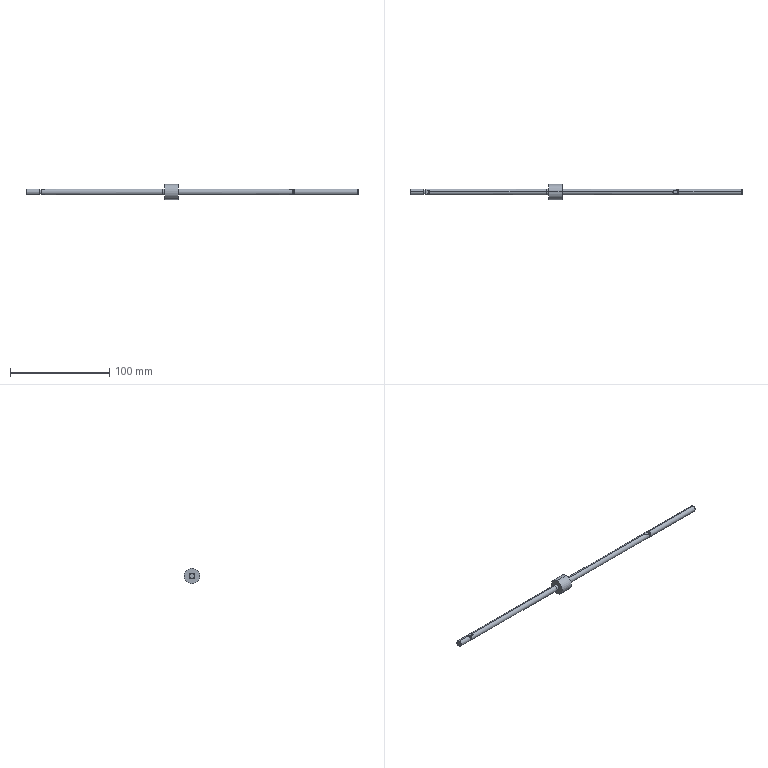Part | SolidWorks | features BaseBody 1 | 1 solid | 41 faces | box 334 x 15.5 x 15.5 mm | volume 11530 mm3 | plane 17 | cylinder 16 | cone 8 | commonest cylinder face diameters 6 x8 4.8 x4 5.8 x2 15.5 x2
STEP:
#1=CARTESIAN_POINT('',(99.1,0.,3.));
#2=VERTEX_POINT('',#1);
#3=CARTESIAN_POINT('',(99.1,0.,-3.));
#4=VERTEX_POINT('',#3);
#5=CARTESIAN_POINT('',(99.1,0.,0.));
#6=DIRECTION('',(-1.,0.,0.));
#7=DIRECTION('',(0.,0.,1.));
#8=AXIS2_PLACEMENT_3D('',#5,#6,#7);
#9=CIRCLE('',#8,3.);
#10=EDGE_CURVE('',#2,#4,#9,.T.);
#11=ORIENTED_EDGE('',*,*,#10,.T.);
#12=CARTESIAN_POINT('',(-18.5,0.,-3.));
#13=VERTEX_POINT('',#12);
#14=CARTESIAN_POINT('',(115.,0.,-3.));
#15=DIRECTION('',(-1.,0.,0.));
#16=VECTOR('',#15,1000.);
#17=LINE('',#14,#16);
#18=EDGE_CURVE('',#4,#13,#17,.T.);
#19=ORIENTED_EDGE('',*,*,#18,.T.);
#20=CARTESIAN_POINT('',(-19.,1.658,-2.5));
#21=VERTEX_POINT('',#20);
#22=CARTESIAN_POINT('',(-18.5,0.,-3.));
#23=CARTESIAN_POINT('',(-18.5,0.5942,-3.));
#24=CARTESIAN_POINT('',(-18.672,1.163,-2.828));
#25=CARTESIAN_POINT('',(-19.,1.658,-2.5));
#26=(BOUNDED_CURVE()B_SPLINE_CURVE(3,(#22,#23,#24,#25),.UNSPECIFIED.,.F.,.F.)B_SPLINE_CURVE_WITH_KNOTS((4,4),(3.142,3.727),.UNSPECIFIED.)CURVE()GEOMETRIC_REPRESENTATION_ITEM()RATIONAL_B_SPLINE_CURVE((1.,0.9716,0.9716,1.))REPRESENTATION_ITEM(''));
#27=EDGE_CURVE('',#13,#21,#26,.T.);
#28=ORIENTED_EDGE('',*,*,#27,.T.);
#29=CARTESIAN_POINT('',(-22.,1.658,-2.5));
#30=VERTEX_POINT('',#29);
#31=CARTESIAN_POINT('',(115.,1.658,-2.5));
#32=DIRECTION('',(-1.,0.,0.));
#33=VECTOR('',#32,1000.);
#34=LINE('',#31,#33);
#35=EDGE_CURVE('',#21,#30,#34,.T.);
#36=ORIENTED_EDGE('',*,*,#35,.T.);
#37=CARTESIAN_POINT('',(-22.,1.658,2.5));
#38=VERTEX_POINT('',#37);
#39=CARTESIAN_POINT('',(-22.,0.,0.));
#40=DIRECTION('',(1.,0.,0.));
#41=DIRECTION('',(0.,0.,1.));
#42=AXIS2_PLACEMENT_3D('',#39,#40,#41);
#43=CIRCLE('',#42,3.);
#44=EDGE_CURVE('',#30,#38,#43,.T.);
#45=ORIENTED_EDGE('',*,*,#44,.T.);
#46=CARTESIAN_POINT('',(-19.,1.658,2.5));
#47=VERTEX_POINT('',#46);
#48=CARTESIAN_POINT('',(115.,1.658,2.5));
#49=DIRECTION('',(1.,0.,0.));
#50=VECTOR('',#49,1000.);
#51=LINE('',#48,#50);
#52=EDGE_CURVE('',#38,#47,#51,.T.);
#53=ORIENTED_EDGE('',*,*,#52,.T.);
#54=CARTESIAN_POINT('',(-18.5,0.,3.));
#55=VERTEX_POINT('',#54);
#56=CARTESIAN_POINT('',(-19.,1.658,2.5));
#57=CARTESIAN_POINT('',(-18.672,1.163,2.828));
#58=CARTESIAN_POINT('',(-18.5,0.5942,3.));
#59=CARTESIAN_POINT('',(-18.5,0.,3.));
#60=(BOUNDED_CURVE()B_SPLINE_CURVE(3,(#56,#57,#58,#59),.UNSPECIFIED.,.F.,.T.)B_SPLINE_CURVE_WITH_KNOTS((4,4),(2.556,3.142),.UNSPECIFIED.)CURVE()GEOMETRIC_REPRESENTATION_ITEM()RATIONAL_B_SPLINE_CURVE((1.,0.9716,0.9716,1.))REPRESENTATION_ITEM(''));
#61=EDGE_CURVE('',#47,#55,#60,.T.);
#62=ORIENTED_EDGE('',*,*,#61,.T.);
#63=CARTESIAN_POINT('',(115.,0.,3.));
#64=DIRECTION('',(-1.,0.,0.));
#65=VECTOR('',#64,1000.);
#66=LINE('',#63,#65);
#67=EDGE_CURVE('',#2,#55,#66,.T.);
#68=ORIENTED_EDGE('',*,*,#67,.F.);
#69=EDGE_LOOP('',(#11,#19,#28,#36,#45,#53,#62,#68));
#70=FACE_OUTER_BOUND('',#69,.T.);
#71=CARTESIAN_POINT('',(115.,0.,0.));
#72=DIRECTION('',(-1.,0.,0.));
#73=DIRECTION('',(0.,0.,1.));
#74=AXIS2_PLACEMENT_3D('',#71,#72,#73);
#75=CYLINDRICAL_SURFACE('',#74,3.);
#76=ADVANCED_FACE('',(#70),#75,.T.);
#77=CARTESIAN_POINT('',(-22.6,0.,-2.4));
#78=VERTEX_POINT('',#77);
#79=CARTESIAN_POINT('',(-22.6,0.,2.4));
#80=VERTEX_POINT('',#79);
#81=CARTESIAN_POINT('',(-22.6,0.,0.));
#82=DIRECTION('',(1.,0.,0.));
#83=DIRECTION('',(0.,0.,-1.));
#84=AXIS2_PLACEMENT_3D('',#81,#82,#83);
#85=CIRCLE('',#84,2.4);
#86=EDGE_CURVE('',#78,#80,#85,.T.);
#87=ORIENTED_EDGE('',*,*,#86,.T.);
#88=CARTESIAN_POINT('',(-22.46,0.,2.54));
#89=VERTEX_POINT('',#88);
#90=CARTESIAN_POINT('',(-22.,0.,3.));
#91=DIRECTION('',(0.7071,0.,0.7071));
#92=VECTOR('',#91,1000.);
#93=LINE('',#90,#92);
#94=EDGE_CURVE('',#80,#89,#93,.T.);
#95=ORIENTED_EDGE('',*,*,#94,.T.);
#96=CARTESIAN_POINT('',(-22.46,0.449,2.5));
#97=VERTEX_POINT('',#96);
#98=CARTESIAN_POINT('',(-22.46,0.,0.));
#99=DIRECTION('',(-1.,0.,0.));
#100=DIRECTION('',(0.,0.,-1.));
#101=AXIS2_PLACEMENT_3D('',#98,#99,#100);
#102=CIRCLE('',#101,2.54);
#103=EDGE_CURVE('',#89,#97,#102,.T.);
#104=ORIENTED_EDGE('',*,*,#103,.T.);
#105=CARTESIAN_POINT('',(-22.,1.658,2.5));
#106=CARTESIAN_POINT('',(-22.211,1.277,2.5));
#107=CARTESIAN_POINT('',(-22.384,0.8814,2.5));
#108=CARTESIAN_POINT('',(-22.46,0.449,2.5));
#109=B_SPLINE_CURVE_WITH_KNOTS('',3,(#105,#106,#107,#108),.UNSPECIFIED.,.F.,.F.,(4,4),(0.,0.001294),.UNSPECIFIED.);
#110=EDGE_CURVE('',#38,#97,#109,.T.);
#111=ORIENTED_EDGE('',*,*,#110,.F.);
#112=ORIENTED_EDGE('',*,*,#44,.F.);
#113=CARTESIAN_POINT('',(-22.46,0.449,-2.5));
#114=VERTEX_POINT('',#113);
#115=CARTESIAN_POINT('',(-22.,1.658,-2.5));
#116=CARTESIAN_POINT('',(-22.211,1.277,-2.5));
#117=CARTESIAN_POINT('',(-22.384,0.8814,-2.5));
#118=CARTESIAN_POINT('',(-22.46,0.449,-2.5));
#119=B_SPLINE_CURVE_WITH_KNOTS('',3,(#115,#116,#117,#118),.UNSPECIFIED.,.F.,.F.,(4,4),(0.,0.001294),.UNSPECIFIED.);
#120=EDGE_CURVE('',#30,#114,#119,.T.);
#121=ORIENTED_EDGE('',*,*,#120,.T.);
#122=CARTESIAN_POINT('',(-22.46,0.,-2.54));
#123=VERTEX_POINT('',#122);
#124=CARTESIAN_POINT('',(-22.46,0.,0.));
#125=DIRECTION('',(-1.,0.,0.));
#126=DIRECTION('',(0.,0.,-1.));
#127=AXIS2_PLACEMENT_3D('',#124,#125,#126);
#128=CIRCLE('',#127,2.54);
#129=EDGE_CURVE('',#114,#123,#128,.T.);
#130=ORIENTED_EDGE('',*,*,#129,.T.);
#131=CARTESIAN_POINT('',(-22.,0.,-3.));
#132=DIRECTION('',(0.7071,0.,-0.7071));
#133=VECTOR('',#132,1000.);
#134=LINE('',#131,#133);
#135=EDGE_CURVE('',#78,#123,#134,.T.);
#136=ORIENTED_EDGE('',*,*,#135,.F.);
#137=EDGE_LOOP('',(#87,#95,#104,#111,#112,#121,#130,#136));
#138=FACE_OUTER_BOUND('',#137,.T.);
#139=CARTESIAN_POINT('',(-22.,0.,0.));
#140=DIRECTION('',(1.,0.,0.));
#141=DIRECTION('',(0.,0.,-1.));
#142=AXIS2_PLACEMENT_3D('',#139,#140,#141);
#143=CONICAL_SURFACE('',#142,3.,0.7854);
#144=ADVANCED_FACE('',(#138),#143,.T.);
#145=ORIENTED_EDGE('',*,*,#86,.F.);
#146=CARTESIAN_POINT('',(-24.,0.,-2.4));
#147=VERTEX_POINT('',#146);
#148=CARTESIAN_POINT('',(115.,0.,-2.4));
#149=DIRECTION('',(-1.,0.,0.));
#150=VECTOR('',#149,1000.);
#151=LINE('',#148,#150);
#152=EDGE_CURVE('',#78,#147,#151,.T.);
#153=ORIENTED_EDGE('',*,*,#152,.T.);
#154=CARTESIAN_POINT('',(-24.,0.,2.4));
#155=VERTEX_POINT('',#154);
#156=CARTESIAN_POINT('',(-24.,0.,0.));
#157=DIRECTION('',(1.,0.,0.));
#158=DIRECTION('',(0.,0.,1.));
#159=AXIS2_PLACEMENT_3D('',#156,#157,#158);
#160=CIRCLE('',#159,2.4);
#161=EDGE_CURVE('',#147,#155,#160,.T.);
#162=ORIENTED_EDGE('',*,*,#161,.T.);
#163=CARTESIAN_POINT('',(115.,0.,2.4));
#164=DIRECTION('',(-1.,0.,0.));
#165=VECTOR('',#164,1000.);
#166=LINE('',#163,#165);
#167=EDGE_CURVE('',#80,#155,#166,.T.);
#168=ORIENTED_EDGE('',*,*,#167,.F.);
#169=EDGE_LOOP('',(#145,#153,#162,#168));
#170=FACE_OUTER_BOUND('',#169,.T.);
#171=CARTESIAN_POINT('',(115.,0.,0.));
#172=DIRECTION('',(-1.,0.,0.));
#173=DIRECTION('',(0.,0.,1.));
#174=AXIS2_PLACEMENT_3D('',#171,#172,#173);
#175=CYLINDRICAL_SURFACE('',#174,2.4);
#176=ADVANCED_FACE('',(#170),#175,.T.);
#177=CARTESIAN_POINT('',(101.6,0.,2.9));
#178=VERTEX_POINT('',#177);
#179=CARTESIAN_POINT('',(101.6,0.,-2.9));
#180=VERTEX_POINT('',#179);
#181=CARTESIAN_POINT('',(101.6,0.,0.));
#182=DIRECTION('',(-1.,0.,0.));
#183=DIRECTION('',(0.,0.,1.));
#184=AXIS2_PLACEMENT_3D('',#181,#182,#183);
#185=CIRCLE('',#184,2.9);
#186=EDGE_CURVE('',#178,#180,#185,.T.);
#187=ORIENTED_EDGE('',*,*,#186,.T.);
#188=CARTESIAN_POINT('',(99.1,0.,-2.9));
#189=VERTEX_POINT('',#188);
#190=CARTESIAN_POINT('',(115.,0.,-2.9));
#191=DIRECTION('',(-1.,0.,0.));
#192=VECTOR('',#191,1000.);
#193=LINE('',#190,#192);
#194=EDGE_CURVE('',#180,#189,#193,.T.);
#195=ORIENTED_EDGE('',*,*,#194,.T.);
#196=CARTESIAN_POINT('',(99.1,0.,2.9));
#197=VERTEX_POINT('',#196);
#198=CARTESIAN_POINT('',(99.1,0.,0.));
#199=DIRECTION('',(1.,0.,0.));
#200=DIRECTION('',(0.,0.,1.));
#201=AXIS2_PLACEMENT_3D('',#198,#199,#200);
#202=CIRCLE('',#201,2.9);
#203=EDGE_CURVE('',#189,#197,#202,.T.);
#204=ORIENTED_EDGE('',*,*,#203,.T.);
#205=CARTESIAN_POINT('',(115.,0.,2.9));
#206=DIRECTION('',(-1.,0.,0.));
#207=VECTOR('',#206,1000.);
#208=LINE('',#205,#207);
#209=EDGE_CURVE('',#178,#197,#208,.T.);
#210=ORIENTED_EDGE('',*,*,#209,.F.);
#211=EDGE_LOOP('',(#187,#195,#204,#210));
#212=FACE_OUTER_BOUND('',#211,.T.);
#213=CARTESIAN_POINT('',(115.,0.,0.));
#214=DIRECTION('',(-1.,0.,0.));
#215=DIRECTION('',(0.,0.,1.));
#216=AXIS2_PLACEMENT_3D('',#213,#214,#215);
#217=CYLINDRICAL_SURFACE('',#216,2.9);
#218=ADVANCED_FACE('',(#212),#217,.T.);
#219=CARTESIAN_POINT('',(-24.,0.,3.));
#220=VERTEX_POINT('',#219);
#221=CARTESIAN_POINT('',(-24.,0.,-3.));
#222=VERTEX_POINT('',#221);
#223=CARTESIAN_POINT('',(-24.,0.,0.));
#224=DIRECTION('',(-1.,0.,0.));
#225=DIRECTION('',(0.,0.,1.));
#226=AXIS2_PLACEMENT_3D('',#223,#224,#225);
#227=CIRCLE('',#226,3.);
#228=EDGE_CURVE('',#220,#222,#227,.T.);
#229=ORIENTED_EDGE('',*,*,#228,.T.);
#230=CARTESIAN_POINT('',(-37.387,0.,-3.));
#231=VERTEX_POINT('',#230);
#232=CARTESIAN_POINT('',(115.,0.,-3.));
#233=DIRECTION('',(-1.,0.,0.));
#234=VECTOR('',#233,1000.);
#235=LINE('',#232,#234);
#236=EDGE_CURVE('',#222,#231,#235,.T.);
#237=ORIENTED_EDGE('',*,*,#236,.T.);
#238=CARTESIAN_POINT('',(-37.387,0.,3.));
#239=VERTEX_POINT('',#238);
#240=CARTESIAN_POINT('',(-37.387,0.,0.));
#241=DIRECTION('',(1.,0.,0.));
#242=DIRECTION('',(0.,0.,1.));
#243=AXIS2_PLACEMENT_3D('',#240,#241,#242);
#244=CIRCLE('',#243,3.);
#245=EDGE_CURVE('',#231,#239,#244,.T.);
#246=ORIENTED_EDGE('',*,*,#245,.T.);
#247=CARTESIAN_POINT('',(115.,0.,3.));
#248=DIRECTION('',(-1.,0.,0.));
#249=VECTOR('',#248,1000.);
#250=LINE('',#247,#249);
#251=EDGE_CURVE('',#220,#239,#250,.T.);
#252=ORIENTED_EDGE('',*,*,#251,.F.);
#253=EDGE_LOOP('',(#229,#237,#246,#252));
#254=FACE_OUTER_BOUND('',#253,.T.);
#255=CARTESIAN_POINT('',(115.,0.,0.));
#256=DIRECTION('',(-1.,0.,0.));
#257=DIRECTION('',(0.,0.,1.));
#258=AXIS2_PLACEMENT_3D('',#255,#256,#257);
#259=CYLINDRICAL_SURFACE('',#258,3.);
#260=ADVANCED_FACE('',(#254),#259,.T.);
#261=CARTESIAN_POINT('',(115.,0.,7.75));
#262=VERTEX_POINT('',#261);
#263=CARTESIAN_POINT('',(115.,0.,-7.75));
#264=VERTEX_POINT('',#263);
#265=CARTESIAN_POINT('',(115.,0.,0.));
#266=DIRECTION('',(-1.,0.,0.));
#267=DIRECTION('',(0.,0.,1.));
#268=AXIS2_PLACEMENT_3D('',#265,#266,#267);
#269=CIRCLE('',#268,7.75);
#270=EDGE_CURVE('',#262,#264,#269,.T.);
#271=ORIENTED_EDGE('',*,*,#270,.T.);
#272=CARTESIAN_POINT('',(101.6,0.,-7.75));
#273=VERTEX_POINT('',#272);
#274=CARTESIAN_POINT('',(115.,0.,-7.75));
#275=DIRECTION('',(-1.,0.,0.));
#276=VECTOR('',#275,1000.);
#277=LINE('',#274,#276);
#278=EDGE_CURVE('',#264,#273,#277,.T.);
#279=ORIENTED_EDGE('',*,*,#278,.T.);
#280=CARTESIAN_POINT('',(101.6,0.,7.75));
#281=VERTEX_POINT('',#280);
#282=CARTESIAN_POINT('',(101.6,0.,0.));
#283=DIRECTION('',(1.,0.,0.));
#284=DIRECTION('',(0.,0.,1.));
#285=AXIS2_PLACEMENT_3D('',#282,#283,#284);
#286=CIRCLE('',#285,7.75);
#287=EDGE_CURVE('',#273,#281,#286,.T.);
#288=ORIENTED_EDGE('',*,*,#287,.T.);
#289=CARTESIAN_POINT('',(115.,0.,7.75));
#290=DIRECTION('',(-1.,0.,0.));
#291=VECTOR('',#290,1000.);
#292=LINE('',#289,#291);
#293=EDGE_CURVE('',#262,#281,#292,.T.);
#294=ORIENTED_EDGE('',*,*,#293,.F.);
#295=EDGE_LOOP('',(#271,#279,#288,#294));
#296=FACE_OUTER_BOUND('',#295,.T.);
#297=CARTESIAN_POINT('',(115.,0.,0.));
#298=DIRECTION('',(-1.,0.,0.));
#299=DIRECTION('',(0.,0.,1.));
#300=AXIS2_PLACEMENT_3D('',#297,#298,#299);
#301=CYLINDRICAL_SURFACE('',#300,7.75);
#302=ADVANCED_FACE('',(#296),#301,.T.);
#303=CARTESIAN_POINT('',(-38.,0.,-2.387));
#304=VERTEX_POINT('',#303);
#305=CARTESIAN_POINT('',(-38.,0.,2.387));
#306=VERTEX_POINT('',#305);
#307=CARTESIAN_POINT('',(-38.,0.,0.));
#308=DIRECTION('',(1.,0.,0.));
#309=DIRECTION('',(0.,0.,-1.));
#310=AXIS2_PLACEMENT_3D('',#307,#308,#309);
#311=CIRCLE('',#310,2.387);
#312=EDGE_CURVE('',#304,#306,#311,.T.);
#313=ORIENTED_EDGE('',*,*,#312,.T.);
#314=CARTESIAN_POINT('',(-37.387,0.,3.));
#315=DIRECTION('',(0.7071,0.,0.7071));
#316=VECTOR('',#315,1000.);
#317=LINE('',#314,#316);
#318=EDGE_CURVE('',#306,#239,#317,.T.);
#319=ORIENTED_EDGE('',*,*,#318,.T.);
#320=ORIENTED_EDGE('',*,*,#245,.F.);
#321=CARTESIAN_POINT('',(-37.387,0.,-3.));
#322=DIRECTION('',(0.7071,0.,-0.7071));
#323=VECTOR('',#322,1000.);
#324=LINE('',#321,#323);
#325=EDGE_CURVE('',#304,#231,#324,.T.);
#326=ORIENTED_EDGE('',*,*,#325,.F.);
#327=EDGE_LOOP('',(#313,#319,#320,#326));
#328=FACE_OUTER_BOUND('',#327,.T.);
#329=CARTESIAN_POINT('',(-37.387,0.,0.));
#330=DIRECTION('',(1.,0.,0.));
#331=DIRECTION('',(0.,0.,-1.));
#332=AXIS2_PLACEMENT_3D('',#329,#330,#331);
#333=CONICAL_SURFACE('',#332,3.,0.7854);
#334=ADVANCED_FACE('',(#328),#333,.T.);
#335=CARTESIAN_POINT('',(227.,1.658,-2.5));
#336=VERTEX_POINT('',#335);
#337=CARTESIAN_POINT('',(226.5,0.,-3.));
#338=VERTEX_POINT('',#337);
#339=CARTESIAN_POINT('',(227.,1.658,-2.5));
#340=CARTESIAN_POINT('',(226.672,1.163,-2.828));
#341=CARTESIAN_POINT('',(226.5,0.5942,-3.));
#342=CARTESIAN_POINT('',(226.5,0.,-3.));
#343=(BOUNDED_CURVE()B_SPLINE_CURVE(3,(#339,#340,#341,#342),.UNSPECIFIED.,.F.,.F.)B_SPLINE_CURVE_WITH_KNOTS((4,4),(5.697,6.283),.UNSPECIFIED.)CURVE()GEOMETRIC_REPRESENTATION_ITEM()RATIONAL_B_SPLINE_CURVE((1.,0.9716,0.9716,1.))REPRESENTATION_ITEM(''));
#344=EDGE_CURVE('',#336,#338,#343,.T.);
#345=ORIENTED_EDGE('',*,*,#344,.T.);
#346=CARTESIAN_POINT('',(115.,0.,-3.));
#347=VERTEX_POINT('',#346);
#348=CARTESIAN_POINT('',(296.,0.,-3.));
#349=DIRECTION('',(-1.,0.,0.));
#350=VECTOR('',#349,1000.);
#351=LINE('',#348,#350);
#352=EDGE_CURVE('',#338,#347,#351,.T.);
#353=ORIENTED_EDGE('',*,*,#352,.T.);
#354=CARTESIAN_POINT('',(115.,0.,3.));
#355=VERTEX_POINT('',#354);
#356=CARTESIAN_POINT('',(115.,0.,0.));
#357=DIRECTION('',(1.,0.,0.));
#358=DIRECTION('',(0.,0.,1.));
#359=AXIS2_PLACEMENT_3D('',#356,#357,#358);
#360=CIRCLE('',#359,3.);
#361=EDGE_CURVE('',#347,#355,#360,.T.);
#362=ORIENTED_EDGE('',*,*,#361,.T.);
#363=CARTESIAN_POINT('',(226.5,0.,3.));
#364=VERTEX_POINT('',#363);
#365=CARTESIAN_POINT('',(296.,0.,3.));
#366=DIRECTION('',(-1.,0.,0.));
#367=VECTOR('',#366,1000.);
#368=LINE('',#365,#367);
#369=EDGE_CURVE('',#364,#355,#368,.T.);
#370=ORIENTED_EDGE('',*,*,#369,.F.);
#371=CARTESIAN_POINT('',(227.,1.658,2.5));
#372=VERTEX_POINT('',#371);
#373=CARTESIAN_POINT('',(226.5,0.,3.));
#374=CARTESIAN_POINT('',(226.5,0.5942,3.));
#375=CARTESIAN_POINT('',(226.672,1.163,2.828));
#376=CARTESIAN_POINT('',(227.,1.658,2.5));
#377=(BOUNDED_CURVE()B_SPLINE_CURVE(3,(#373,#374,#375,#376),.UNSPECIFIED.,.F.,.F.)B_SPLINE_CURVE_WITH_KNOTS((4,4),(0.,0.5857),.UNSPECIFIED.)CURVE()GEOMETRIC_REPRESENTATION_ITEM()RATIONAL_B_SPLINE_CURVE((1.,0.9716,0.9716,1.))REPRESENTATION_ITEM(''));
#378=EDGE_CURVE('',#364,#372,#377,.T.);
#379=ORIENTED_EDGE('',*,*,#378,.T.);
#380=CARTESIAN_POINT('',(230.4,1.658,2.5));
#381=VERTEX_POINT('',#380);
#382=CARTESIAN_POINT('',(296.,1.658,2.5));
#383=DIRECTION('',(1.,0.,0.));
#384=VECTOR('',#383,1000.);
#385=LINE('',#382,#384);
#386=EDGE_CURVE('',#372,#381,#385,.T.);
#387=ORIENTED_EDGE('',*,*,#386,.T.);
#388=CARTESIAN_POINT('',(230.4,1.658,-2.5));
#389=VERTEX_POINT('',#388);
#390=CARTESIAN_POINT('',(230.4,0.,0.));
#391=DIRECTION('',(-1.,0.,0.));
#392=DIRECTION('',(0.,0.,1.));
#393=AXIS2_PLACEMENT_3D('',#390,#391,#392);
#394=CIRCLE('',#393,3.);
#395=EDGE_CURVE('',#381,#389,#394,.T.);
#396=ORIENTED_EDGE('',*,*,#395,.T.);
#397=CARTESIAN_POINT('',(296.,1.658,-2.5));
#398=DIRECTION('',(-1.,0.,0.));
#399=VECTOR('',#398,1000.);
#400=LINE('',#397,#399);
#401=EDGE_CURVE('',#389,#336,#400,.T.);
#402=ORIENTED_EDGE('',*,*,#401,.T.);
#403=EDGE_LOOP('',(#345,#353,#362,#370,#379,#387,#396,#402));
#404=FACE_OUTER_BOUND('',#403,.T.);
#405=CARTESIAN_POINT('',(296.,0.,0.));
#406=DIRECTION('',(-1.,0.,0.));
#407=DIRECTION('',(0.,0.,1.));
#408=AXIS2_PLACEMENT_3D('',#405,#406,#407);
#409=CYLINDRICAL_SURFACE('',#408,3.);
#410=ADVANCED_FACE('',(#404),#409,.T.);
#411=CARTESIAN_POINT('',(231.,0.,2.4));
#412=VERTEX_POINT('',#411);
#413=CARTESIAN_POINT('',(231.,0.,-2.4));
#414=VERTEX_POINT('',#413);
#415=CARTESIAN_POINT('',(231.,0.,0.));
#416=DIRECTION('',(-1.,0.,0.));
#417=DIRECTION('',(0.,0.,1.));
#418=AXIS2_PLACEMENT_3D('',#415,#416,#417);
#419=CIRCLE('',#418,2.4);
#420=EDGE_CURVE('',#412,#414,#419,.T.);
#421=ORIENTED_EDGE('',*,*,#420,.T.);
#422=CARTESIAN_POINT('',(230.9,0.,-2.5));
#423=VERTEX_POINT('',#422);
#424=CARTESIAN_POINT('',(230.4,0.,-3.));
#425=DIRECTION('',(-0.7071,0.,-0.7071));
#426=VECTOR('',#425,1000.);
#427=LINE('',#424,#426);
#428=EDGE_CURVE('',#414,#423,#427,.T.);
#429=ORIENTED_EDGE('',*,*,#428,.T.);
#430=CARTESIAN_POINT('',(230.9,0.,-2.5));
#431=CARTESIAN_POINT('',(230.9,0.1452,-2.5));
#432=CARTESIAN_POINT('',(230.887,0.2917,-2.5));
#433=CARTESIAN_POINT('',(230.837,0.5812,-2.5));
#434=CARTESIAN_POINT('',(230.801,0.7221,-2.5));
#435=CARTESIAN_POINT('',(230.666,1.136,-2.5));
#436=CARTESIAN_POINT('',(230.542,1.402,-2.5));
#437=CARTESIAN_POINT('',(230.4,1.658,-2.5));
#438=B_SPLINE_CURVE_WITH_KNOTS('',3,(#430,#431,#432,#433,#434,#435,#436,#437),.UNSPECIFIED.,.F.,.F.,(4,2,2,4),(0.001744,0.002179,0.002615,0.003485),.UNSPECIFIED.);
#439=EDGE_CURVE('',#423,#389,#438,.T.);
#440=ORIENTED_EDGE('',*,*,#439,.T.);
#441=ORIENTED_EDGE('',*,*,#395,.F.);
#442=CARTESIAN_POINT('',(230.9,0.,2.5));
#443=VERTEX_POINT('',#442);
#444=CARTESIAN_POINT('',(230.9,0.,2.5));
#445=CARTESIAN_POINT('',(230.9,0.1452,2.5));
#446=CARTESIAN_POINT('',(230.887,0.2917,2.5));
#447=CARTESIAN_POINT('',(230.837,0.5812,2.5));
#448=CARTESIAN_POINT('',(230.801,0.7221,2.5));
#449=CARTESIAN_POINT('',(230.666,1.136,2.5));
#450=CARTESIAN_POINT('',(230.542,1.402,2.5));
#451=CARTESIAN_POINT('',(230.4,1.658,2.5));
#452=B_SPLINE_CURVE_WITH_KNOTS('',3,(#444,#445,#446,#447,#448,#449,#450,#451),.UNSPECIFIED.,.F.,.F.,(4,2,2,4),(0.001744,0.002179,0.002615,0.003485),.UNSPECIFIED.);
#453=EDGE_CURVE('',#443,#381,#452,.T.);
#454=ORIENTED_EDGE('',*,*,#453,.F.);
#455=CARTESIAN_POINT('',(230.4,0.,3.));
#456=DIRECTION('',(-0.7071,0.,0.7071));
#457=VECTOR('',#456,1000.);
#458=LINE('',#455,#457);
#459=EDGE_CURVE('',#412,#443,#458,.T.);
#460=ORIENTED_EDGE('',*,*,#459,.F.);
#461=EDGE_LOOP('',(#421,#429,#440,#441,#454,#460));
#462=FACE_OUTER_BOUND('',#461,.T.);
#463=CARTESIAN_POINT('',(230.4,0.,0.));
#464=DIRECTION('',(-1.,0.,0.));
#465=DIRECTION('',(0.,0.,1.));
#466=AXIS2_PLACEMENT_3D('',#463,#464,#465);
#467=CONICAL_SURFACE('',#466,3.,0.7854);
#468=ADVANCED_FACE('',(#462),#467,.T.);
#469=CARTESIAN_POINT('',(232.5,0.,2.4));
#470=VERTEX_POINT('',#469);
#471=CARTESIAN_POINT('',(232.5,0.,-2.4));
#472=VERTEX_POINT('',#471);
#473=CARTESIAN_POINT('',(232.5,0.,0.));
#474=DIRECTION('',(-1.,0.,0.));
#475=DIRECTION('',(0.,0.,1.));
#476=AXIS2_PLACEMENT_3D('',#473,#474,#475);
#477=CIRCLE('',#476,2.4);
#478=EDGE_CURVE('',#470,#472,#477,.T.);
#479=ORIENTED_EDGE('',*,*,#478,.T.);
#480=CARTESIAN_POINT('',(296.,0.,-2.4));
#481=DIRECTION('',(-1.,0.,0.));
#482=VECTOR('',#481,1000.);
#483=LINE('',#480,#482);
#484=EDGE_CURVE('',#472,#414,#483,.T.);
#485=ORIENTED_EDGE('',*,*,#484,.T.);
#486=ORIENTED_EDGE('',*,*,#420,.F.);
#487=CARTESIAN_POINT('',(296.,0.,2.4));
#488=DIRECTION('',(-1.,0.,0.));
#489=VECTOR('',#488,1000.);
#490=LINE('',#487,#489);
#491=EDGE_CURVE('',#470,#412,#490,.T.);
#492=ORIENTED_EDGE('',*,*,#491,.F.);
#493=EDGE_LOOP('',(#479,#485,#486,#492));
#494=FACE_OUTER_BOUND('',#493,.T.);
#495=CARTESIAN_POINT('',(296.,0.,0.));
#496=DIRECTION('',(-1.,0.,0.));
#497=DIRECTION('',(0.,0.,1.));
#498=AXIS2_PLACEMENT_3D('',#495,#496,#497);
#499=CYLINDRICAL_SURFACE('',#498,2.4);
#500=ADVANCED_FACE('',(#494),#499,.T.);
#501=CARTESIAN_POINT('',(295.387,0.,3.));
#502=VERTEX_POINT('',#501);
#503=CARTESIAN_POINT('',(295.387,0.,-3.));
#504=VERTEX_POINT('',#503);
#505=CARTESIAN_POINT('',(295.387,0.,0.));
#506=DIRECTION('',(-1.,0.,0.));
#507=DIRECTION('',(0.,0.,1.));
#508=AXIS2_PLACEMENT_3D('',#505,#506,#507);
#509=CIRCLE('',#508,3.);
#510=EDGE_CURVE('',#502,#504,#509,.T.);
#511=ORIENTED_EDGE('',*,*,#510,.T.);
#512=CARTESIAN_POINT('',(232.5,0.,-3.));
#513=VERTEX_POINT('',#512);
#514=CARTESIAN_POINT('',(296.,0.,-3.));
#515=DIRECTION('',(-1.,0.,0.));
#516=VECTOR('',#515,1000.);
#517=LINE('',#514,#516);
#518=EDGE_CURVE('',#504,#513,#517,.T.);
#519=ORIENTED_EDGE('',*,*,#518,.T.);
#520=CARTESIAN_POINT('',(232.5,0.,3.));
#521=VERTEX_POINT('',#520);
#522=CARTESIAN_POINT('',(232.5,0.,0.));
#523=DIRECTION('',(1.,0.,0.));
#524=DIRECTION('',(0.,0.,1.));
#525=AXIS2_PLACEMENT_3D('',#522,#523,#524);
#526=CIRCLE('',#525,3.);
#527=EDGE_CURVE('',#513,#521,#526,.T.);
#528=ORIENTED_EDGE('',*,*,#527,.T.);
#529=CARTESIAN_POINT('',(296.,0.,3.));
#530=DIRECTION('',(-1.,0.,0.));
#531=VECTOR('',#530,1000.);
#532=LINE('',#529,#531);
#533=EDGE_CURVE('',#502,#521,#532,.T.);
#534=ORIENTED_EDGE('',*,*,#533,.F.);
#535=EDGE_LOOP('',(#511,#519,#528,#534));
#536=FACE_OUTER_BOUND('',#535,.T.);
#537=CARTESIAN_POINT('',(296.,0.,0.));
#538=DIRECTION('',(-1.,0.,0.));
#539=DIRECTION('',(0.,0.,1.));
#540=AXIS2_PLACEMENT_3D('',#537,#538,#539);
#541=CYLINDRICAL_SURFACE('',#540,3.);
#542=ADVANCED_FACE('',(#536),#541,.T.);
#543=CARTESIAN_POINT('',(296.,0.,2.386));
#544=VERTEX_POINT('',#543);
#545=CARTESIAN_POINT('',(296.,0.,-2.386));
#546=VERTEX_POINT('',#545);
#547=CARTESIAN_POINT('',(296.,0.,0.));
#548=DIRECTION('',(-1.,0.,0.));
#549=DIRECTION('',(0.,0.,1.));
#550=AXIS2_PLACEMENT_3D('',#547,#548,#549);
#551=CIRCLE('',#550,2.386);
#552=EDGE_CURVE('',#544,#546,#551,.T.);
#553=ORIENTED_EDGE('',*,*,#552,.T.);
#554=CARTESIAN_POINT('',(295.386,0.,-3.));
#555=DIRECTION('',(-0.7071,0.,-0.7071));
#556=VECTOR('',#555,1000.);
#557=LINE('',#554,#556);
#558=EDGE_CURVE('',#546,#504,#557,.T.);
#559=ORIENTED_EDGE('',*,*,#558,.T.);
#560=ORIENTED_EDGE('',*,*,#510,.F.);
#561=CARTESIAN_POINT('',(295.386,0.,3.));
#562=DIRECTION('',(-0.7071,0.,0.7071));
#563=VECTOR('',#562,1000.);
#564=LINE('',#561,#563);
#565=EDGE_CURVE('',#544,#502,#564,.T.);
#566=ORIENTED_EDGE('',*,*,#565,.F.);
#567=EDGE_LOOP('',(#553,#559,#560,#566));
#568=FACE_OUTER_BOUND('',#567,.T.);
#569=CARTESIAN_POINT('',(295.386,0.,0.));
#570=DIRECTION('',(-1.,0.,0.));
#571=DIRECTION('',(0.,0.,1.));
#572=AXIS2_PLACEMENT_3D('',#569,#570,#571);
#573=CONICAL_SURFACE('',#572,3.,0.7854);
#574=ADVANCED_FACE('',(#568),#573,.T.);
#575=ORIENTED_EDGE('',*,*,#18,.F.);
#576=CARTESIAN_POINT('',(99.1,0.,0.));
#577=DIRECTION('',(-1.,0.,0.));
#578=DIRECTION('',(0.,0.,1.));
#579=AXIS2_PLACEMENT_3D('',#576,#577,#578);
#580=CIRCLE('',#579,3.);
#581=EDGE_CURVE('',#4,#2,#580,.T.);
#582=ORIENTED_EDGE('',*,*,#581,.T.);
#583=ORIENTED_EDGE('',*,*,#67,.T.);
#584=CARTESIAN_POINT('',(-19.,-1.658,2.5));
#585=VERTEX_POINT('',#584);
#586=CARTESIAN_POINT('',(-18.5,0.,3.));
#587=CARTESIAN_POINT('',(-18.5,-0.5942,3.));
#588=CARTESIAN_POINT('',(-18.672,-1.163,2.828));
#589=CARTESIAN_POINT('',(-19.,-1.658,2.5));
#590=(BOUNDED_CURVE()B_SPLINE_CURVE(3,(#586,#587,#588,#589),.UNSPECIFIED.,.F.,.F.)B_SPLINE_CURVE_WITH_KNOTS((4,4),(3.142,3.727),.UNSPECIFIED.)CURVE()GEOMETRIC_REPRESENTATION_ITEM()RATIONAL_B_SPLINE_CURVE((1.,0.9716,0.9716,1.))REPRESENTATION_ITEM(''));
#591=EDGE_CURVE('',#55,#585,#590,.T.);
#592=ORIENTED_EDGE('',*,*,#591,.T.);
#593=CARTESIAN_POINT('',(-22.,-1.658,2.5));
#594=VERTEX_POINT('',#593);
#595=CARTESIAN_POINT('',(115.,-1.658,2.5));
#596=DIRECTION('',(-1.,0.,0.));
#597=VECTOR('',#596,1000.);
#598=LINE('',#595,#597);
#599=EDGE_CURVE('',#585,#594,#598,.T.);
#600=ORIENTED_EDGE('',*,*,#599,.T.);
#601=CARTESIAN_POINT('',(-22.,-1.658,-2.5));
#602=VERTEX_POINT('',#601);
#603=CARTESIAN_POINT('',(-22.,0.,0.));
#604=DIRECTION('',(1.,0.,0.));
#605=DIRECTION('',(0.,0.,1.));
#606=AXIS2_PLACEMENT_3D('',#603,#604,#605);
#607=CIRCLE('',#606,3.);
#608=EDGE_CURVE('',#594,#602,#607,.T.);
#609=ORIENTED_EDGE('',*,*,#608,.T.);
#610=CARTESIAN_POINT('',(-19.,-1.658,-2.5));
#611=VERTEX_POINT('',#610);
#612=CARTESIAN_POINT('',(115.,-1.658,-2.5));
#613=DIRECTION('',(1.,0.,0.));
#614=VECTOR('',#613,1000.);
#615=LINE('',#612,#614);
#616=EDGE_CURVE('',#602,#611,#615,.T.);
#617=ORIENTED_EDGE('',*,*,#616,.T.);
#618=CARTESIAN_POINT('',(-19.,-1.658,-2.5));
#619=CARTESIAN_POINT('',(-18.672,-1.163,-2.828));
#620=CARTESIAN_POINT('',(-18.5,-0.5942,-3.));
#621=CARTESIAN_POINT('',(-18.5,0.,-3.));
#622=(BOUNDED_CURVE()B_SPLINE_CURVE(3,(#618,#619,#620,#621),.UNSPECIFIED.,.F.,.F.)B_SPLINE_CURVE_WITH_KNOTS((4,4),(2.556,3.142),.UNSPECIFIED.)CURVE()GEOMETRIC_REPRESENTATION_ITEM()RATIONAL_B_SPLINE_CURVE((1.,0.9716,0.9716,1.))REPRESENTATION_ITEM(''));
#623=EDGE_CURVE('',#611,#13,#622,.T.);
#624=ORIENTED_EDGE('',*,*,#623,.T.);
#625=EDGE_LOOP('',(#575,#582,#583,#592,#600,#609,#617,#624));
#626=FACE_OUTER_BOUND('',#625,.T.);
#627=CARTESIAN_POINT('',(115.,0.,0.));
#628=DIRECTION('',(-1.,0.,0.));
#629=DIRECTION('',(0.,0.,1.));
#630=AXIS2_PLACEMENT_3D('',#627,#628,#629);
#631=CYLINDRICAL_SURFACE('',#630,3.);
#632=ADVANCED_FACE('',(#626),#631,.T.);
#633=ORIENTED_EDGE('',*,*,#61,.F.);
#634=CARTESIAN_POINT('',(-19.,6.,2.5));
#635=DIRECTION('',(0.,-1.,0.));
#636=VECTOR('',#635,1000.);
#637=LINE('',#634,#636);
#638=EDGE_CURVE('',#47,#585,#637,.T.);
#639=ORIENTED_EDGE('',*,*,#638,.T.);
#640=ORIENTED_EDGE('',*,*,#591,.F.);
#641=EDGE_LOOP('',(#633,#639,#640));
#642=FACE_OUTER_BOUND('',#641,.T.);
#643=CARTESIAN_POINT('',(-16.5,6.,5.));
#644=DIRECTION('',(-0.7071,0.,0.7071));
#645=DIRECTION('',(0.7071,0.,0.7071));
#646=AXIS2_PLACEMENT_3D('',#643,#644,#645);
#647=PLANE('',#646);
#648=ADVANCED_FACE('',(#642),#647,.T.);
#649=ORIENTED_EDGE('',*,*,#110,.T.);
#650=CARTESIAN_POINT('',(-22.46,-0.449,2.5));
#651=VERTEX_POINT('',#650);
#652=CARTESIAN_POINT('',(-22.46,6.,2.5));
#653=DIRECTION('',(0.,-1.,0.));
#654=VECTOR('',#653,1000.);
#655=LINE('',#652,#654);
#656=EDGE_CURVE('',#97,#651,#655,.T.);
#657=ORIENTED_EDGE('',*,*,#656,.T.);
#658=CARTESIAN_POINT('',(-22.46,-0.449,2.5));
#659=CARTESIAN_POINT('',(-22.384,-0.8798,2.5));
#660=CARTESIAN_POINT('',(-22.211,-1.277,2.5));
#661=CARTESIAN_POINT('',(-22.,-1.658,2.5));
#662=B_SPLINE_CURVE_WITH_KNOTS('',3,(#658,#659,#660,#661),.UNSPECIFIED.,.F.,.F.,(4,4),(0.,0.001294),.UNSPECIFIED.);
#663=EDGE_CURVE('',#651,#594,#662,.T.);
#664=ORIENTED_EDGE('',*,*,#663,.T.);
#665=ORIENTED_EDGE('',*,*,#599,.F.);
#666=ORIENTED_EDGE('',*,*,#638,.F.);
#667=ORIENTED_EDGE('',*,*,#52,.F.);
#668=EDGE_LOOP('',(#649,#657,#664,#665,#666,#667));
#669=FACE_OUTER_BOUND('',#668,.T.);
#670=CARTESIAN_POINT('',(-19.,6.,2.5));
#671=DIRECTION('',(0.,0.,1.));
#672=DIRECTION('',(1.,0.,0.));
#673=AXIS2_PLACEMENT_3D('',#670,#671,#672);
#674=PLANE('',#673);
#675=ADVANCED_FACE('',(#669),#674,.T.);
#676=ORIENTED_EDGE('',*,*,#94,.F.);
#677=CARTESIAN_POINT('',(-22.6,0.,0.));
#678=DIRECTION('',(1.,0.,0.));
#679=DIRECTION('',(0.,0.,-1.));
#680=AXIS2_PLACEMENT_3D('',#677,#678,#679);
#681=CIRCLE('',#680,2.4);
#682=EDGE_CURVE('',#80,#78,#681,.T.);
#683=ORIENTED_EDGE('',*,*,#682,.T.);
#684=ORIENTED_EDGE('',*,*,#135,.T.);
#685=CARTESIAN_POINT('',(-22.46,-0.449,-2.5));
#686=VERTEX_POINT('',#685);
#687=CARTESIAN_POINT('',(-22.46,0.,0.));
#688=DIRECTION('',(-1.,0.,0.));
#689=DIRECTION('',(0.,0.,-1.));
#690=AXIS2_PLACEMENT_3D('',#687,#688,#689);
#691=CIRCLE('',#690,2.54);
#692=EDGE_CURVE('',#123,#686,#691,.T.);
#693=ORIENTED_EDGE('',*,*,#692,.T.);
#694=CARTESIAN_POINT('',(-22.46,-0.449,-2.5));
#695=CARTESIAN_POINT('',(-22.384,-0.8798,-2.5));
#696=CARTESIAN_POINT('',(-22.211,-1.277,-2.5));
#697=CARTESIAN_POINT('',(-22.,-1.658,-2.5));
#698=B_SPLINE_CURVE_WITH_KNOTS('',3,(#694,#695,#696,#697),.UNSPECIFIED.,.F.,.F.,(4,4),(0.,0.001294),.UNSPECIFIED.);
#699=EDGE_CURVE('',#686,#602,#698,.T.);
#700=ORIENTED_EDGE('',*,*,#699,.T.);
#701=ORIENTED_EDGE('',*,*,#608,.F.);
#702=ORIENTED_EDGE('',*,*,#663,.F.);
#703=CARTESIAN_POINT('',(-22.46,0.,0.));
#704=DIRECTION('',(-1.,0.,0.));
#705=DIRECTION('',(0.,0.,-1.));
#706=AXIS2_PLACEMENT_3D('',#703,#704,#705);
#707=CIRCLE('',#706,2.54);
#708=EDGE_CURVE('',#651,#89,#707,.T.);
#709=ORIENTED_EDGE('',*,*,#708,.T.);
#710=EDGE_LOOP('',(#676,#683,#684,#693,#700,#701,#702,#709));
#711=FACE_OUTER_BOUND('',#710,.T.);
#712=CARTESIAN_POINT('',(-22.,0.,0.));
#713=DIRECTION('',(1.,0.,0.));
#714=DIRECTION('',(0.,0.,-1.));
#715=AXIS2_PLACEMENT_3D('',#712,#713,#714);
#716=CONICAL_SURFACE('',#715,3.,0.7854);
#717=ADVANCED_FACE('',(#711),#716,.T.);
#718=ORIENTED_EDGE('',*,*,#699,.F.);
#719=CARTESIAN_POINT('',(-22.46,6.,-2.5));
#720=DIRECTION('',(0.,1.,0.));
#721=VECTOR('',#720,1000.);
#722=LINE('',#719,#721);
#723=EDGE_CURVE('',#686,#114,#722,.T.);
#724=ORIENTED_EDGE('',*,*,#723,.T.);
#725=ORIENTED_EDGE('',*,*,#120,.F.);
#726=ORIENTED_EDGE('',*,*,#35,.F.);
#727=CARTESIAN_POINT('',(-19.,6.,-2.5));
#728=DIRECTION('',(0.,-1.,0.));
#729=VECTOR('',#728,1000.);
#730=LINE('',#727,#729);
#731=EDGE_CURVE('',#21,#611,#730,.T.);
#732=ORIENTED_EDGE('',*,*,#731,.T.);
#733=ORIENTED_EDGE('',*,*,#616,.F.);
#734=EDGE_LOOP('',(#718,#724,#725,#726,#732,#733));
#735=FACE_OUTER_BOUND('',#734,.T.);
#736=CARTESIAN_POINT('',(-22.46,6.,-2.5));
#737=DIRECTION('',(0.,0.,-1.));
#738=DIRECTION('',(-1.,0.,0.));
#739=AXIS2_PLACEMENT_3D('',#736,#737,#738);
#740=PLANE('',#739);
#741=ADVANCED_FACE('',(#735),#740,.T.);
#742=ORIENTED_EDGE('',*,*,#623,.F.);
#743=ORIENTED_EDGE('',*,*,#731,.F.);
#744=ORIENTED_EDGE('',*,*,#27,.F.);
#745=EDGE_LOOP('',(#742,#743,#744));
#746=FACE_OUTER_BOUND('',#745,.T.);
#747=CARTESIAN_POINT('',(-19.,6.,-2.5));
#748=DIRECTION('',(-0.7071,0.,-0.7071));
#749=DIRECTION('',(-0.7071,0.,0.7071));
#750=AXIS2_PLACEMENT_3D('',#747,#748,#749);
#751=PLANE('',#750);
#752=ADVANCED_FACE('',(#746),#751,.T.);
#753=ORIENTED_EDGE('',*,*,#10,.F.);
#754=ORIENTED_EDGE('',*,*,#581,.F.);
#755=EDGE_LOOP('',(#753,#754));
#756=FACE_OUTER_BOUND('',#755,.T.);
#757=CARTESIAN_POINT('',(99.1,0.,0.));
#758=DIRECTION('',(1.,0.,0.));
#759=DIRECTION('',(0.,0.,1.));
#760=AXIS2_PLACEMENT_3D('',#757,#758,#759);
#761=CIRCLE('',#760,2.9);
#762=EDGE_CURVE('',#197,#189,#761,.T.);
#763=ORIENTED_EDGE('',*,*,#762,.F.);
#764=ORIENTED_EDGE('',*,*,#203,.F.);
#765=EDGE_LOOP('',(#763,#764));
#766=FACE_BOUND('',#765,.T.);
#767=CARTESIAN_POINT('',(99.1,3.,0.));
#768=DIRECTION('',(-1.,0.,0.));
#769=DIRECTION('',(0.,0.,1.));
#770=AXIS2_PLACEMENT_3D('',#767,#768,#769);
#771=PLANE('',#770);
#772=ADVANCED_FACE('',(#756,#766),#771,.F.);
#773=ORIENTED_EDGE('',*,*,#708,.F.);
#774=ORIENTED_EDGE('',*,*,#656,.F.);
#775=ORIENTED_EDGE('',*,*,#103,.F.);
#776=EDGE_LOOP('',(#773,#774,#775));
#777=FACE_OUTER_BOUND('',#776,.T.);
#778=CARTESIAN_POINT('',(-22.46,6.,2.5));
#779=DIRECTION('',(1.,0.,0.));
#780=DIRECTION('',(0.,0.,-1.));
#781=AXIS2_PLACEMENT_3D('',#778,#779,#780);
#782=PLANE('',#781);
#783=ADVANCED_FACE('',(#777),#782,.T.);
#784=ORIENTED_EDGE('',*,*,#152,.F.);
#785=ORIENTED_EDGE('',*,*,#682,.F.);
#786=ORIENTED_EDGE('',*,*,#167,.T.);
#787=CARTESIAN_POINT('',(-24.,0.,0.));
#788=DIRECTION('',(1.,0.,0.));
#789=DIRECTION('',(0.,0.,1.));
#790=AXIS2_PLACEMENT_3D('',#787,#788,#789);
#791=CIRCLE('',#790,2.4);
#792=EDGE_CURVE('',#155,#147,#791,.T.);
#793=ORIENTED_EDGE('',*,*,#792,.T.);
#794=EDGE_LOOP('',(#784,#785,#786,#793));
#795=FACE_OUTER_BOUND('',#794,.T.);
#796=CARTESIAN_POINT('',(115.,0.,0.));
#797=DIRECTION('',(-1.,0.,0.));
#798=DIRECTION('',(0.,0.,1.));
#799=AXIS2_PLACEMENT_3D('',#796,#797,#798);
#800=CYLINDRICAL_SURFACE('',#799,2.4);
#801=ADVANCED_FACE('',(#795),#800,.T.);
#802=ORIENTED_EDGE('',*,*,#129,.F.);
#803=ORIENTED_EDGE('',*,*,#723,.F.);
#804=ORIENTED_EDGE('',*,*,#692,.F.);
#805=EDGE_LOOP('',(#802,#803,#804));
#806=FACE_OUTER_BOUND('',#805,.T.);
#807=CARTESIAN_POINT('',(-22.46,6.,-5.));
#808=DIRECTION('',(1.,0.,0.));
#809=DIRECTION('',(0.,0.,-1.));
#810=AXIS2_PLACEMENT_3D('',#807,#808,#809);
#811=PLANE('',#810);
#812=ADVANCED_FACE('',(#806),#811,.T.);
#813=ORIENTED_EDGE('',*,*,#194,.F.);
#814=CARTESIAN_POINT('',(101.6,0.,0.));
#815=DIRECTION('',(-1.,0.,0.));
#816=DIRECTION('',(0.,0.,1.));
#817=AXIS2_PLACEMENT_3D('',#814,#815,#816);
#818=CIRCLE('',#817,2.9);
#819=EDGE_CURVE('',#180,#178,#818,.T.);
#820=ORIENTED_EDGE('',*,*,#819,.T.);
#821=ORIENTED_EDGE('',*,*,#209,.T.);
#822=ORIENTED_EDGE('',*,*,#762,.T.);
#823=EDGE_LOOP('',(#813,#820,#821,#822));
#824=FACE_OUTER_BOUND('',#823,.T.);
#825=CARTESIAN_POINT('',(115.,0.,0.));
#826=DIRECTION('',(-1.,0.,0.));
#827=DIRECTION('',(0.,0.,1.));
#828=AXIS2_PLACEMENT_3D('',#825,#826,#827);
#829=CYLINDRICAL_SURFACE('',#828,2.9);
#830=ADVANCED_FACE('',(#824),#829,.T.);
#831=ORIENTED_EDGE('',*,*,#228,.F.);
#832=CARTESIAN_POINT('',(-24.,0.,0.));
#833=DIRECTION('',(-1.,0.,0.));
#834=DIRECTION('',(0.,0.,1.));
#835=AXIS2_PLACEMENT_3D('',#832,#833,#834);
#836=CIRCLE('',#835,3.);
#837=EDGE_CURVE('',#222,#220,#836,.T.);
#838=ORIENTED_EDGE('',*,*,#837,.F.);
#839=EDGE_LOOP('',(#831,#838));
#840=FACE_OUTER_BOUND('',#839,.T.);
#841=ORIENTED_EDGE('',*,*,#792,.F.);
#842=ORIENTED_EDGE('',*,*,#161,.F.);
#843=EDGE_LOOP('',(#841,#842));
#844=FACE_BOUND('',#843,.T.);
#845=CARTESIAN_POINT('',(-24.,3.,0.));
#846=DIRECTION('',(-1.,0.,0.));
#847=DIRECTION('',(0.,0.,1.));
#848=AXIS2_PLACEMENT_3D('',#845,#846,#847);
#849=PLANE('',#848);
#850=ADVANCED_FACE('',(#840,#844),#849,.F.);
#851=ORIENTED_EDGE('',*,*,#186,.F.);
#852=ORIENTED_EDGE('',*,*,#819,.F.);
#853=EDGE_LOOP('',(#851,#852));
#854=FACE_BOUND('',#853,.T.);
#855=CARTESIAN_POINT('',(101.6,0.,0.));
#856=DIRECTION('',(1.,0.,0.));
#857=DIRECTION('',(0.,0.,1.));
#858=AXIS2_PLACEMENT_3D('',#855,#856,#857);
#859=CIRCLE('',#858,7.75);
#860=EDGE_CURVE('',#281,#273,#859,.T.);
#861=ORIENTED_EDGE('',*,*,#860,.F.);
#862=ORIENTED_EDGE('',*,*,#287,.F.);
#863=EDGE_LOOP('',(#861,#862));
#864=FACE_OUTER_BOUND('',#863,.T.);
#865=CARTESIAN_POINT('',(101.6,2.9,0.));
#866=DIRECTION('',(1.,0.,0.));
#867=DIRECTION('',(0.,0.,-1.));
#868=AXIS2_PLACEMENT_3D('',#865,#866,#867);
#869=PLANE('',#868);
#870=ADVANCED_FACE('',(#854,#864),#869,.F.);
#871=ORIENTED_EDGE('',*,*,#236,.F.);
#872=ORIENTED_EDGE('',*,*,#837,.T.);
#873=ORIENTED_EDGE('',*,*,#251,.T.);
#874=CARTESIAN_POINT('',(-37.387,0.,0.));
#875=DIRECTION('',(1.,0.,0.));
#876=DIRECTION('',(0.,0.,1.));
#877=AXIS2_PLACEMENT_3D('',#874,#875,#876);
#878=CIRCLE('',#877,3.);
#879=EDGE_CURVE('',#239,#231,#878,.T.);
#880=ORIENTED_EDGE('',*,*,#879,.T.);
#881=EDGE_LOOP('',(#871,#872,#873,#880));
#882=FACE_OUTER_BOUND('',#881,.T.);
#883=CARTESIAN_POINT('',(115.,0.,0.));
#884=DIRECTION('',(-1.,0.,0.));
#885=DIRECTION('',(0.,0.,1.));
#886=AXIS2_PLACEMENT_3D('',#883,#884,#885);
#887=CYLINDRICAL_SURFACE('',#886,3.);
#888=ADVANCED_FACE('',(#882),#887,.T.);
#889=ORIENTED_EDGE('',*,*,#278,.F.);
#890=CARTESIAN_POINT('',(115.,0.,0.));
#891=DIRECTION('',(-1.,0.,0.));
#892=DIRECTION('',(0.,0.,1.));
#893=AXIS2_PLACEMENT_3D('',#890,#891,#892);
#894=CIRCLE('',#893,7.75);
#895=EDGE_CURVE('',#264,#262,#894,.T.);
#896=ORIENTED_EDGE('',*,*,#895,.T.);
#897=ORIENTED_EDGE('',*,*,#293,.T.);
#898=ORIENTED_EDGE('',*,*,#860,.T.);
#899=EDGE_LOOP('',(#889,#896,#897,#898));
#900=FACE_OUTER_BOUND('',#899,.T.);
#901=CARTESIAN_POINT('',(115.,0.,0.));
#902=DIRECTION('',(-1.,0.,0.));
#903=DIRECTION('',(0.,0.,1.));
#904=AXIS2_PLACEMENT_3D('',#901,#902,#903);
#905=CYLINDRICAL_SURFACE('',#904,7.75);
#906=ADVANCED_FACE('',(#900),#905,.T.);
#907=ORIENTED_EDGE('',*,*,#318,.F.);
#908=CARTESIAN_POINT('',(-38.,0.,0.));
#909=DIRECTION('',(1.,0.,0.));
#910=DIRECTION('',(0.,0.,-1.));
#911=AXIS2_PLACEMENT_3D('',#908,#909,#910);
#912=CIRCLE('',#911,2.387);
#913=EDGE_CURVE('',#306,#304,#912,.T.);
#914=ORIENTED_EDGE('',*,*,#913,.T.);
#915=ORIENTED_EDGE('',*,*,#325,.T.);
#916=ORIENTED_EDGE('',*,*,#879,.F.);
#917=EDGE_LOOP('',(#907,#914,#915,#916));
#918=FACE_OUTER_BOUND('',#917,.T.);
#919=CARTESIAN_POINT('',(-37.387,0.,0.));
#920=DIRECTION('',(1.,0.,0.));
#921=DIRECTION('',(0.,0.,-1.));
#922=AXIS2_PLACEMENT_3D('',#919,#920,#921);
#923=CONICAL_SURFACE('',#922,3.,0.7854);
#924=ADVANCED_FACE('',(#918),#923,.T.);
#925=ORIENTED_EDGE('',*,*,#270,.F.);
#926=ORIENTED_EDGE('',*,*,#895,.F.);
#927=EDGE_LOOP('',(#925,#926));
#928=FACE_OUTER_BOUND('',#927,.T.);
#929=CARTESIAN_POINT('',(115.,0.,0.));
#930=DIRECTION('',(1.,0.,0.));
#931=DIRECTION('',(0.,0.,1.));
#932=AXIS2_PLACEMENT_3D('',#929,#930,#931);
#933=CIRCLE('',#932,3.);
#934=EDGE_CURVE('',#355,#347,#933,.T.);
#935=ORIENTED_EDGE('',*,*,#934,.F.);
#936=ORIENTED_EDGE('',*,*,#361,.F.);
#937=EDGE_LOOP('',(#935,#936));
#938=FACE_BOUND('',#937,.T.);
#939=CARTESIAN_POINT('',(115.,7.75,0.));
#940=DIRECTION('',(-1.,0.,0.));
#941=DIRECTION('',(0.,0.,1.));
#942=AXIS2_PLACEMENT_3D('',#939,#940,#941);
#943=PLANE('',#942);
#944=ADVANCED_FACE('',(#928,#938),#943,.F.);
#945=ORIENTED_EDGE('',*,*,#312,.F.);
#946=ORIENTED_EDGE('',*,*,#913,.F.);
#947=EDGE_LOOP('',(#945,#946));
#948=FACE_OUTER_BOUND('',#947,.T.);
#949=CARTESIAN_POINT('',(-38.,0.,0.));
#950=DIRECTION('',(1.,0.,0.));
#951=DIRECTION('',(0.,0.,-1.));
#952=AXIS2_PLACEMENT_3D('',#949,#950,#951);
#953=PLANE('',#952);
#954=ADVANCED_FACE('',(#948),#953,.F.);
#955=ORIENTED_EDGE('',*,*,#352,.F.);
#956=CARTESIAN_POINT('',(227.,-1.658,-2.5));
#957=VERTEX_POINT('',#956);
#958=CARTESIAN_POINT('',(226.5,0.,-3.));
#959=CARTESIAN_POINT('',(226.5,-0.5942,-3.));
#960=CARTESIAN_POINT('',(226.672,-1.163,-2.828));
#961=CARTESIAN_POINT('',(227.,-1.658,-2.5));
#962=(BOUNDED_CURVE()B_SPLINE_CURVE(3,(#958,#959,#960,#961),.UNSPECIFIED.,.F.,.F.)B_SPLINE_CURVE_WITH_KNOTS((4,4),(0.,0.5857),.UNSPECIFIED.)CURVE()GEOMETRIC_REPRESENTATION_ITEM()RATIONAL_B_SPLINE_CURVE((1.,0.9716,0.9716,1.))REPRESENTATION_ITEM(''));
#963=EDGE_CURVE('',#338,#957,#962,.T.);
#964=ORIENTED_EDGE('',*,*,#963,.T.);
#965=CARTESIAN_POINT('',(230.4,-1.658,-2.5));
#966=VERTEX_POINT('',#965);
#967=CARTESIAN_POINT('',(296.,-1.658,-2.5));
#968=DIRECTION('',(1.,0.,0.));
#969=VECTOR('',#968,1000.);
#970=LINE('',#967,#969);
#971=EDGE_CURVE('',#957,#966,#970,.T.);
#972=ORIENTED_EDGE('',*,*,#971,.T.);
#973=CARTESIAN_POINT('',(230.4,-1.658,2.5));
#974=VERTEX_POINT('',#973);
#975=CARTESIAN_POINT('',(230.4,0.,0.));
#976=DIRECTION('',(-1.,0.,0.));
#977=DIRECTION('',(0.,0.,1.));
#978=AXIS2_PLACEMENT_3D('',#975,#976,#977);
#979=CIRCLE('',#978,3.);
#980=EDGE_CURVE('',#966,#974,#979,.T.);
#981=ORIENTED_EDGE('',*,*,#980,.T.);
#982=CARTESIAN_POINT('',(227.,-1.658,2.5));
#983=VERTEX_POINT('',#982);
#984=CARTESIAN_POINT('',(296.,-1.658,2.5));
#985=DIRECTION('',(-1.,0.,0.));
#986=VECTOR('',#985,1000.);
#987=LINE('',#984,#986);
#988=EDGE_CURVE('',#974,#983,#987,.T.);
#989=ORIENTED_EDGE('',*,*,#988,.T.);
#990=CARTESIAN_POINT('',(227.,-1.658,2.5));
#991=CARTESIAN_POINT('',(226.672,-1.163,2.828));
#992=CARTESIAN_POINT('',(226.5,-0.5942,3.));
#993=CARTESIAN_POINT('',(226.5,0.,3.));
#994=(BOUNDED_CURVE()B_SPLINE_CURVE(3,(#990,#991,#992,#993),.UNSPECIFIED.,.F.,.F.)B_SPLINE_CURVE_WITH_KNOTS((4,4),(5.697,6.283),.UNSPECIFIED.)CURVE()GEOMETRIC_REPRESENTATION_ITEM()RATIONAL_B_SPLINE_CURVE((1.,0.9716,0.9716,1.))REPRESENTATION_ITEM(''));
#995=EDGE_CURVE('',#983,#364,#994,.T.);
#996=ORIENTED_EDGE('',*,*,#995,.T.);
#997=ORIENTED_EDGE('',*,*,#369,.T.);
#998=ORIENTED_EDGE('',*,*,#934,.T.);
#999=EDGE_LOOP('',(#955,#964,#972,#981,#989,#996,#997,#998));
#1000=FACE_OUTER_BOUND('',#999,.T.);
#1001=CARTESIAN_POINT('',(296.,0.,0.));
#1002=DIRECTION('',(-1.,0.,0.));
#1003=DIRECTION('',(0.,0.,1.));
#1004=AXIS2_PLACEMENT_3D('',#1001,#1002,#1003);
#1005=CYLINDRICAL_SURFACE('',#1004,3.);
#1006=ADVANCED_FACE('',(#1000),#1005,.T.);
#1007=ORIENTED_EDGE('',*,*,#386,.F.);
#1008=CARTESIAN_POINT('',(227.,6.,2.5));
#1009=DIRECTION('',(0.,-1.,0.));
#1010=VECTOR('',#1009,1000.);
#1011=LINE('',#1008,#1010);
#1012=EDGE_CURVE('',#372,#983,#1011,.T.);
#1013=ORIENTED_EDGE('',*,*,#1012,.T.);
#1014=ORIENTED_EDGE('',*,*,#988,.F.);
#1015=CARTESIAN_POINT('',(230.4,-1.658,2.5));
#1016=CARTESIAN_POINT('',(230.542,-1.402,2.5));
#1017=CARTESIAN_POINT('',(230.666,-1.138,2.5));
#1018=CARTESIAN_POINT('',(230.846,-0.5844,2.5));
#1019=CARTESIAN_POINT('',(230.9,-0.2908,2.5));
#1020=CARTESIAN_POINT('',(230.9,0.,2.5));
#1021=B_SPLINE_CURVE_WITH_KNOTS('',3,(#1015,#1016,#1017,#1018,#1019,#1020),.UNSPECIFIED.,.F.,.F.,(4,2,4),(0.,0.000872,0.001744),.UNSPECIFIED.);
#1022=EDGE_CURVE('',#974,#443,#1021,.T.);
#1023=ORIENTED_EDGE('',*,*,#1022,.T.);
#1024=ORIENTED_EDGE('',*,*,#453,.T.);
#1025=EDGE_LOOP('',(#1007,#1013,#1014,#1023,#1024));
#1026=FACE_OUTER_BOUND('',#1025,.T.);
#1027=CARTESIAN_POINT('',(231.,6.,2.5));
#1028=DIRECTION('',(0.,0.,1.));
#1029=DIRECTION('',(1.,0.,0.));
#1030=AXIS2_PLACEMENT_3D('',#1027,#1028,#1029);
#1031=PLANE('',#1030);
#1032=ADVANCED_FACE('',(#1026),#1031,.T.);
#1033=ORIENTED_EDGE('',*,*,#995,.F.);
#1034=ORIENTED_EDGE('',*,*,#1012,.F.);
#1035=ORIENTED_EDGE('',*,*,#378,.F.);
#1036=EDGE_LOOP('',(#1033,#1034,#1035));
#1037=FACE_OUTER_BOUND('',#1036,.T.);
#1038=CARTESIAN_POINT('',(227.,6.,2.5));
#1039=DIRECTION('',(0.7071,0.,0.7071));
#1040=DIRECTION('',(0.7071,0.,-0.7071));
#1041=AXIS2_PLACEMENT_3D('',#1038,#1039,#1040);
#1042=PLANE('',#1041);
#1043=ADVANCED_FACE('',(#1037),#1042,.T.);
#1044=ORIENTED_EDGE('',*,*,#428,.F.);
#1045=CARTESIAN_POINT('',(231.,0.,0.));
#1046=DIRECTION('',(-1.,0.,0.));
#1047=DIRECTION('',(0.,0.,1.));
#1048=AXIS2_PLACEMENT_3D('',#1045,#1046,#1047);
#1049=CIRCLE('',#1048,2.4);
#1050=EDGE_CURVE('',#414,#412,#1049,.T.);
#1051=ORIENTED_EDGE('',*,*,#1050,.T.);
#1052=ORIENTED_EDGE('',*,*,#459,.T.);
#1053=ORIENTED_EDGE('',*,*,#1022,.F.);
#1054=ORIENTED_EDGE('',*,*,#980,.F.);
#1055=CARTESIAN_POINT('',(230.4,-1.658,-2.5));
#1056=CARTESIAN_POINT('',(230.542,-1.402,-2.5));
#1057=CARTESIAN_POINT('',(230.666,-1.138,-2.5));
#1058=CARTESIAN_POINT('',(230.846,-0.5844,-2.5));
#1059=CARTESIAN_POINT('',(230.9,-0.2908,-2.5));
#1060=CARTESIAN_POINT('',(230.9,0.,-2.5));
#1061=B_SPLINE_CURVE_WITH_KNOTS('',3,(#1055,#1056,#1057,#1058,#1059,#1060),.UNSPECIFIED.,.F.,.F.,(4,2,4),(0.,0.000872,0.001744),.UNSPECIFIED.);
#1062=EDGE_CURVE('',#966,#423,#1061,.T.);
#1063=ORIENTED_EDGE('',*,*,#1062,.T.);
#1064=EDGE_LOOP('',(#1044,#1051,#1052,#1053,#1054,#1063));
#1065=FACE_OUTER_BOUND('',#1064,.T.);
#1066=CARTESIAN_POINT('',(230.4,0.,0.));
#1067=DIRECTION('',(-1.,0.,0.));
#1068=DIRECTION('',(0.,0.,1.));
#1069=AXIS2_PLACEMENT_3D('',#1066,#1067,#1068);
#1070=CONICAL_SURFACE('',#1069,3.,0.7854);
#1071=ADVANCED_FACE('',(#1065),#1070,.T.);
#1072=ORIENTED_EDGE('',*,*,#971,.F.);
#1073=CARTESIAN_POINT('',(227.,6.,-2.5));
#1074=DIRECTION('',(0.,1.,0.));
#1075=VECTOR('',#1074,1000.);
#1076=LINE('',#1073,#1075);
#1077=EDGE_CURVE('',#957,#336,#1076,.T.);
#1078=ORIENTED_EDGE('',*,*,#1077,.T.);
#1079=ORIENTED_EDGE('',*,*,#401,.F.);
#1080=ORIENTED_EDGE('',*,*,#439,.F.);
#1081=ORIENTED_EDGE('',*,*,#1062,.F.);
#1082=EDGE_LOOP('',(#1072,#1078,#1079,#1080,#1081));
#1083=FACE_OUTER_BOUND('',#1082,.T.);
#1084=CARTESIAN_POINT('',(227.,6.,-2.5));
#1085=DIRECTION('',(0.,0.,-1.));
#1086=DIRECTION('',(-1.,0.,0.));
#1087=AXIS2_PLACEMENT_3D('',#1084,#1085,#1086);
#1088=PLANE('',#1087);
#1089=ADVANCED_FACE('',(#1083),#1088,.T.);
#1090=ORIENTED_EDGE('',*,*,#344,.F.);
#1091=ORIENTED_EDGE('',*,*,#1077,.F.);
#1092=ORIENTED_EDGE('',*,*,#963,.F.);
#1093=EDGE_LOOP('',(#1090,#1091,#1092));
#1094=FACE_OUTER_BOUND('',#1093,.T.);
#1095=CARTESIAN_POINT('',(224.5,6.,-5.));
#1096=DIRECTION('',(0.7071,0.,-0.7071));
#1097=DIRECTION('',(-0.7071,0.,-0.7071));
#1098=AXIS2_PLACEMENT_3D('',#1095,#1096,#1097);
#1099=PLANE('',#1098);
#1100=ADVANCED_FACE('',(#1094),#1099,.T.);
#1101=ORIENTED_EDGE('',*,*,#484,.F.);
#1102=CARTESIAN_POINT('',(232.5,0.,0.));
#1103=DIRECTION('',(-1.,0.,0.));
#1104=DIRECTION('',(0.,0.,1.));
#1105=AXIS2_PLACEMENT_3D('',#1102,#1103,#1104);
#1106=CIRCLE('',#1105,2.4);
#1107=EDGE_CURVE('',#472,#470,#1106,.T.);
#1108=ORIENTED_EDGE('',*,*,#1107,.T.);
#1109=ORIENTED_EDGE('',*,*,#491,.T.);
#1110=ORIENTED_EDGE('',*,*,#1050,.F.);
#1111=EDGE_LOOP('',(#1101,#1108,#1109,#1110));
#1112=FACE_OUTER_BOUND('',#1111,.T.);
#1113=CARTESIAN_POINT('',(296.,0.,0.));
#1114=DIRECTION('',(-1.,0.,0.));
#1115=DIRECTION('',(0.,0.,1.));
#1116=AXIS2_PLACEMENT_3D('',#1113,#1114,#1115);
#1117=CYLINDRICAL_SURFACE('',#1116,2.4);
#1118=ADVANCED_FACE('',(#1112),#1117,.T.);
#1119=ORIENTED_EDGE('',*,*,#478,.F.);
#1120=ORIENTED_EDGE('',*,*,#1107,.F.);
#1121=EDGE_LOOP('',(#1119,#1120));
#1122=FACE_BOUND('',#1121,.T.);
#1123=CARTESIAN_POINT('',(232.5,0.,0.));
#1124=DIRECTION('',(1.,0.,0.));
#1125=DIRECTION('',(0.,0.,1.));
#1126=AXIS2_PLACEMENT_3D('',#1123,#1124,#1125);
#1127=CIRCLE('',#1126,3.);
#1128=EDGE_CURVE('',#521,#513,#1127,.T.);
#1129=ORIENTED_EDGE('',*,*,#1128,.F.);
#1130=ORIENTED_EDGE('',*,*,#527,.F.);
#1131=EDGE_LOOP('',(#1129,#1130));
#1132=FACE_OUTER_BOUND('',#1131,.T.);
#1133=CARTESIAN_POINT('',(232.5,2.4,0.));
#1134=DIRECTION('',(1.,0.,0.));
#1135=DIRECTION('',(0.,0.,-1.));
#1136=AXIS2_PLACEMENT_3D('',#1133,#1134,#1135);
#1137=PLANE('',#1136);
#1138=ADVANCED_FACE('',(#1122,#1132),#1137,.F.);
#1139=ORIENTED_EDGE('',*,*,#518,.F.);
#1140=CARTESIAN_POINT('',(295.387,0.,0.));
#1141=DIRECTION('',(-1.,0.,0.));
#1142=DIRECTION('',(0.,0.,1.));
#1143=AXIS2_PLACEMENT_3D('',#1140,#1141,#1142);
#1144=CIRCLE('',#1143,3.);
#1145=EDGE_CURVE('',#504,#502,#1144,.T.);
#1146=ORIENTED_EDGE('',*,*,#1145,.T.);
#1147=ORIENTED_EDGE('',*,*,#533,.T.);
#1148=ORIENTED_EDGE('',*,*,#1128,.T.);
#1149=EDGE_LOOP('',(#1139,#1146,#1147,#1148));
#1150=FACE_OUTER_BOUND('',#1149,.T.);
#1151=CARTESIAN_POINT('',(296.,0.,0.));
#1152=DIRECTION('',(-1.,0.,0.));
#1153=DIRECTION('',(0.,0.,1.));
#1154=AXIS2_PLACEMENT_3D('',#1151,#1152,#1153);
#1155=CYLINDRICAL_SURFACE('',#1154,3.);
#1156=ADVANCED_FACE('',(#1150),#1155,.T.);
#1157=ORIENTED_EDGE('',*,*,#558,.F.);
#1158=CARTESIAN_POINT('',(296.,0.,0.));
#1159=DIRECTION('',(-1.,0.,0.));
#1160=DIRECTION('',(0.,0.,1.));
#1161=AXIS2_PLACEMENT_3D('',#1158,#1159,#1160);
#1162=CIRCLE('',#1161,2.386);
#1163=EDGE_CURVE('',#546,#544,#1162,.T.);
#1164=ORIENTED_EDGE('',*,*,#1163,.T.);
#1165=ORIENTED_EDGE('',*,*,#565,.T.);
#1166=ORIENTED_EDGE('',*,*,#1145,.F.);
#1167=EDGE_LOOP('',(#1157,#1164,#1165,#1166));
#1168=FACE_OUTER_BOUND('',#1167,.T.);
#1169=CARTESIAN_POINT('',(295.386,0.,0.));
#1170=DIRECTION('',(-1.,0.,0.));
#1171=DIRECTION('',(0.,0.,1.));
#1172=AXIS2_PLACEMENT_3D('',#1169,#1170,#1171);
#1173=CONICAL_SURFACE('',#1172,3.,0.7854);
#1174=ADVANCED_FACE('',(#1168),#1173,.T.);
#1175=ORIENTED_EDGE('',*,*,#552,.F.);
#1176=ORIENTED_EDGE('',*,*,#1163,.F.);
#1177=EDGE_LOOP('',(#1175,#1176));
#1178=FACE_OUTER_BOUND('',#1177,.T.);
#1179=CARTESIAN_POINT('',(296.,2.386,0.));
#1180=DIRECTION('',(-1.,0.,0.));
#1181=DIRECTION('',(0.,0.,1.));
#1182=AXIS2_PLACEMENT_3D('',#1179,#1180,#1181);
#1183=PLANE('',#1182);
#1184=ADVANCED_FACE('',(#1178),#1183,.F.);
#1185=CLOSED_SHELL('',(#76,#144,#176,#218,#260,#302,#334,#410,#468,#500,#542,#574,#632,#648,#675,#717,#741,#752,#772,#783,#801,#812,#830,#850,#870,#888,#906,#924,#944,#954,#1006,#1032,#1043,#1071,#1089,#1100,#1118,#1138,#1156,#1174,#1184));
#1186=MANIFOLD_SOLID_BREP('',#1185);
#1187=CARTESIAN_POINT('',(0.,0.,0.));
#1188=DIRECTION('',(0.,0.,1.));
#1189=DIRECTION('',(1.,0.,0.));
#1190=AXIS2_PLACEMENT_3D('',#1187,#1188,#1189);
#1191=(LENGTH_UNIT()NAMED_UNIT(*)SI_UNIT(.MILLI.,.METRE.));
#1192=UNCERTAINTY_MEASURE_WITH_UNIT(LENGTH_MEASURE(0.00001),#1191,'','');
#1193=(NAMED_UNIT(*)PLANE_ANGLE_UNIT()SI_UNIT($,.RADIAN.));
#1194=(NAMED_UNIT(*)SI_UNIT($,.STERADIAN.)SOLID_ANGLE_UNIT());
#1195=(GEOMETRIC_REPRESENTATION_CONTEXT(3)GLOBAL_UNCERTAINTY_ASSIGNED_CONTEXT((#1192))GLOBAL_UNIT_ASSIGNED_CONTEXT((#1191,#1193,#1194))REPRESENTATION_CONTEXT('',''));
#1196=ADVANCED_BREP_SHAPE_REPRESENTATION('',(#1186,#1190),#1195);